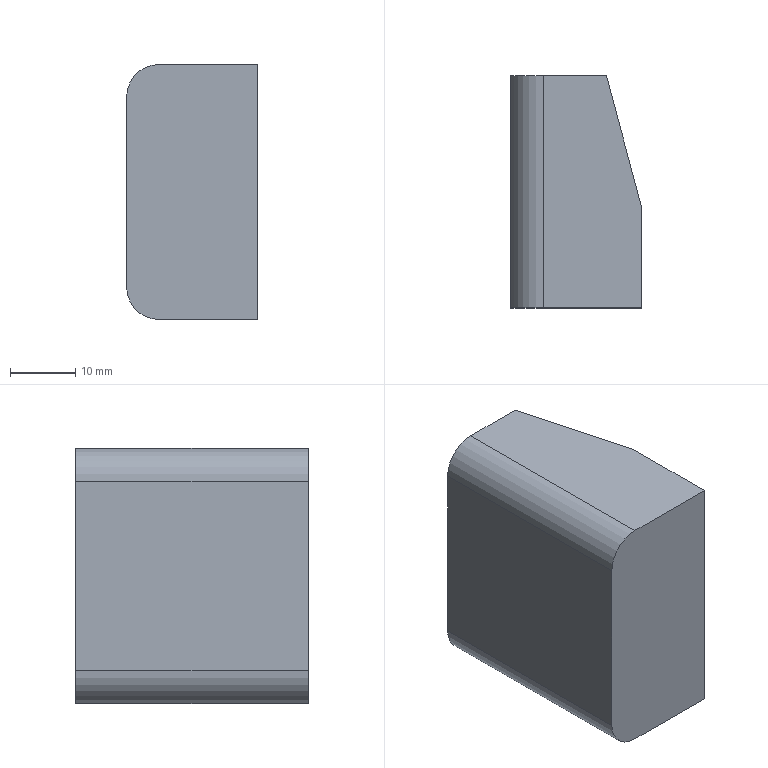Part | STEP file | 1 solid | 9 faces | box 20 x 35.5 x 39 mm | volume 25224 mm3 | plane 7 | cylinder 2 | commonest cylinder face diameters 10 x2
STEP:
#1=CARTESIAN_POINT('',(0.,0.,0.));
#2=DIRECTION('',(0.,0.,1.));
#3=DIRECTION('',(1.,0.,0.));
#4=AXIS2_PLACEMENT_3D('',#1,#2,#3);
#5=CARTESIAN_POINT('',(-257.863,50.,145.951));
#6=VERTEX_POINT('',#5);
#7=CARTESIAN_POINT('',(-252.863,50.,140.951));
#8=VERTEX_POINT('',#7);
#9=CARTESIAN_POINT('',(-252.863,50.,145.951));
#10=DIRECTION('',(0.,-1.,0.));
#11=DIRECTION('',(0.,0.,1.));
#12=AXIS2_PLACEMENT_3D('',#9,#10,#11);
#13=CIRCLE('',#12,5.);
#14=CARTESIAN_POINT('',(-252.863,-7.5,145.951));
#15=DIRECTION('',(0.,-1.,0.));
#16=DIRECTION('',(0.,0.,-1.));
#17=AXIS2_PLACEMENT_3D('',#14,#15,#16);
#18=CYLINDRICAL_SURFACE('',#17,5.);
#19=CARTESIAN_POINT('',(3.142,-57.5));
#20=DIRECTION('',(1.,0.));
#21=VECTOR('',#20,1.);
#22=LINE('',#19,#21);
#23=(GEOMETRIC_REPRESENTATION_CONTEXT(2)PARAMETRIC_REPRESENTATION_CONTEXT()REPRESENTATION_CONTEXT('',''));
#24=DEFINITIONAL_REPRESENTATION('',(#22),#23);
#25=PCURVE('',#18,#24);
#26=CARTESIAN_POINT('',(-72.862,50.,108.53));
#27=DIRECTION('',(0.,1.,0.));
#28=DIRECTION('',(0.,0.,1.));
#29=AXIS2_PLACEMENT_3D('',#26,#27,#28);
#30=PLANE('',#29);
#31=CARTESIAN_POINT('',(42.422,-180.));
#32=CARTESIAN_POINT('',(42.422,-188.66));
#33=CARTESIAN_POINT('',(34.922,-184.33));
#34=CARTESIAN_POINT('',(27.422,-180.));
#35=CARTESIAN_POINT('',(34.922,-175.67));
#36=CARTESIAN_POINT('',(42.422,-171.34));
#37=CARTESIAN_POINT('',(42.422,-180.));
#38=(BOUNDED_CURVE()B_SPLINE_CURVE(2,(#31,#32,#33,#34,#35,#36,#37),.UNSPECIFIED.,.T.,.F.)B_SPLINE_CURVE_WITH_KNOTS((1,2,2,2,2,1),(-2.094,0.,2.094,4.189,6.283,8.378),.UNSPECIFIED.)CURVE()GEOMETRIC_REPRESENTATION_ITEM()RATIONAL_B_SPLINE_CURVE((1.,0.5,1.,0.5,1.,0.5,1.))REPRESENTATION_ITEM(''));
#39=(GEOMETRIC_REPRESENTATION_CONTEXT(2)PARAMETRIC_REPRESENTATION_CONTEXT()REPRESENTATION_CONTEXT('',''));
#40=DEFINITIONAL_REPRESENTATION('',(#38),#39);
#41=PCURVE('',#30,#40);
#42=SURFACE_CURVE('',#13,(#25,#41),.PCURVE_S1.);
#43=EDGE_CURVE('',#6,#8,#42,.T.);
#44=ORIENTED_EDGE('',*,*,#43,.F.);
#45=CARTESIAN_POINT('',(-257.863,85.5,145.951));
#46=VERTEX_POINT('',#45);
#47=CARTESIAN_POINT('',(-257.863,-7.5,145.951));
#48=DIRECTION('',(0.,-1.,0.));
#49=VECTOR('',#48,1.);
#50=LINE('',#47,#49);
#51=CARTESIAN_POINT('',(4.712,0.));
#52=DIRECTION('',(0.,1.));
#53=VECTOR('',#52,1.);
#54=LINE('',#51,#53);
#55=(GEOMETRIC_REPRESENTATION_CONTEXT(2)PARAMETRIC_REPRESENTATION_CONTEXT()REPRESENTATION_CONTEXT('',''));
#56=DEFINITIONAL_REPRESENTATION('',(#54),#55);
#57=PCURVE('',#18,#56);
#58=CARTESIAN_POINT('',(-257.863,-7.5,140.951));
#59=DIRECTION('',(-1.,0.,0.));
#60=DIRECTION('',(0.,0.,1.));
#61=AXIS2_PLACEMENT_3D('',#58,#59,#60);
#62=PLANE('',#61);
#63=CARTESIAN_POINT('',(5.,0.));
#64=DIRECTION('',(0.,-1.));
#65=VECTOR('',#64,1.);
#66=LINE('',#63,#65);
#67=(GEOMETRIC_REPRESENTATION_CONTEXT(2)PARAMETRIC_REPRESENTATION_CONTEXT()REPRESENTATION_CONTEXT('',''));
#68=DEFINITIONAL_REPRESENTATION('',(#66),#67);
#69=PCURVE('',#62,#68);
#70=SURFACE_CURVE('',#50,(#57,#69),.PCURVE_S1.);
#71=EDGE_CURVE('',#46,#6,#70,.T.);
#72=ORIENTED_EDGE('',*,*,#71,.F.);
#73=CARTESIAN_POINT('',(-252.863,85.5,140.951));
#74=VERTEX_POINT('',#73);
#75=CARTESIAN_POINT('',(-252.863,85.5,145.951));
#76=DIRECTION('',(0.,1.,0.));
#77=DIRECTION('',(0.,0.,-1.));
#78=AXIS2_PLACEMENT_3D('',#75,#76,#77);
#79=CIRCLE('',#78,5.);
#80=CARTESIAN_POINT('',(6.283,-93.));
#81=DIRECTION('',(-1.,0.));
#82=VECTOR('',#81,1.);
#83=LINE('',#80,#82);
#84=(GEOMETRIC_REPRESENTATION_CONTEXT(2)PARAMETRIC_REPRESENTATION_CONTEXT()REPRESENTATION_CONTEXT('',''));
#85=DEFINITIONAL_REPRESENTATION('',(#83),#84);
#86=PCURVE('',#18,#85);
#87=CARTESIAN_POINT('',(-72.862,85.5,-363.47));
#88=DIRECTION('',(0.,-1.,0.));
#89=DIRECTION('',(0.,0.,-1.));
#90=AXIS2_PLACEMENT_3D('',#87,#88,#89);
#91=PLANE('',#90);
#92=CARTESIAN_POINT('',(-504.422,-180.));
#93=CARTESIAN_POINT('',(-504.422,-188.66));
#94=CARTESIAN_POINT('',(-511.922,-184.33));
#95=CARTESIAN_POINT('',(-519.422,-180.));
#96=CARTESIAN_POINT('',(-511.922,-175.67));
#97=CARTESIAN_POINT('',(-504.422,-171.34));
#98=CARTESIAN_POINT('',(-504.422,-180.));
#99=(BOUNDED_CURVE()B_SPLINE_CURVE(2,(#92,#93,#94,#95,#96,#97,#98),.UNSPECIFIED.,.T.,.F.)B_SPLINE_CURVE_WITH_KNOTS((1,2,2,2,2,1),(-2.094,0.,2.094,4.189,6.283,8.378),.UNSPECIFIED.)CURVE()GEOMETRIC_REPRESENTATION_ITEM()RATIONAL_B_SPLINE_CURVE((1.,0.5,1.,0.5,1.,0.5,1.))REPRESENTATION_ITEM(''));
#100=(GEOMETRIC_REPRESENTATION_CONTEXT(2)PARAMETRIC_REPRESENTATION_CONTEXT()REPRESENTATION_CONTEXT('',''));
#101=DEFINITIONAL_REPRESENTATION('',(#99),#100);
#102=PCURVE('',#91,#101);
#103=SURFACE_CURVE('',#79,(#86,#102),.PCURVE_S1.);
#104=EDGE_CURVE('',#74,#46,#103,.T.);
#105=ORIENTED_EDGE('',*,*,#104,.F.);
#106=CARTESIAN_POINT('',(-252.863,-7.5,140.951));
#107=DIRECTION('',(0.,1.,0.));
#108=VECTOR('',#107,1.);
#109=LINE('',#106,#108);
#110=CARTESIAN_POINT('',(6.283,0.));
#111=DIRECTION('',(0.,-1.));
#112=VECTOR('',#111,1.);
#113=LINE('',#110,#112);
#114=(GEOMETRIC_REPRESENTATION_CONTEXT(2)PARAMETRIC_REPRESENTATION_CONTEXT()REPRESENTATION_CONTEXT('',''));
#115=DEFINITIONAL_REPRESENTATION('',(#113),#114);
#116=PCURVE('',#18,#115);
#117=CARTESIAN_POINT('',(-240.363,-7.5,140.951));
#118=DIRECTION('',(0.,0.,-1.));
#119=DIRECTION('',(-1.,0.,0.));
#120=AXIS2_PLACEMENT_3D('',#117,#118,#119);
#121=PLANE('',#120);
#122=CARTESIAN_POINT('',(12.5,0.));
#123=DIRECTION('',(0.,1.));
#124=VECTOR('',#123,1.);
#125=LINE('',#122,#124);
#126=(GEOMETRIC_REPRESENTATION_CONTEXT(2)PARAMETRIC_REPRESENTATION_CONTEXT()REPRESENTATION_CONTEXT('',''));
#127=DEFINITIONAL_REPRESENTATION('',(#125),#126);
#128=PCURVE('',#121,#127);
#129=SURFACE_CURVE('',#109,(#116,#128),.PCURVE_S1.);
#130=EDGE_CURVE('',#8,#74,#129,.T.);
#131=ORIENTED_EDGE('',*,*,#130,.F.);
#132=EDGE_LOOP('',(#44,#72,#105,#131));
#133=FACE_BOUND('',#132,.T.);
#134=ADVANCED_FACE('',(#133),#18,.T.);
#135=CARTESIAN_POINT('',(-257.863,50.,174.951));
#136=VERTEX_POINT('',#135);
#137=CARTESIAN_POINT('',(-257.863,50.,140.951));
#138=DIRECTION('',(0.,0.,-1.));
#139=VECTOR('',#138,1.);
#140=LINE('',#137,#139);
#141=CARTESIAN_POINT('',(0.,57.5));
#142=DIRECTION('',(-1.,0.));
#143=VECTOR('',#142,1.);
#144=LINE('',#141,#143);
#145=(GEOMETRIC_REPRESENTATION_CONTEXT(2)PARAMETRIC_REPRESENTATION_CONTEXT()REPRESENTATION_CONTEXT('',''));
#146=DEFINITIONAL_REPRESENTATION('',(#144),#145);
#147=PCURVE('',#62,#146);
#148=CARTESIAN_POINT('',(32.422,-185.));
#149=DIRECTION('',(-1.,0.));
#150=VECTOR('',#149,1.);
#151=LINE('',#148,#150);
#152=(GEOMETRIC_REPRESENTATION_CONTEXT(2)PARAMETRIC_REPRESENTATION_CONTEXT()REPRESENTATION_CONTEXT('',''));
#153=DEFINITIONAL_REPRESENTATION('',(#151),#152);
#154=PCURVE('',#30,#153);
#155=SURFACE_CURVE('',#140,(#147,#154),.PCURVE_S1.);
#156=EDGE_CURVE('',#136,#6,#155,.T.);
#157=ORIENTED_EDGE('',*,*,#156,.F.);
#158=CARTESIAN_POINT('',(-257.863,85.5,174.951));
#159=VERTEX_POINT('',#158);
#160=CARTESIAN_POINT('',(-257.863,-7.5,174.951));
#161=DIRECTION('',(0.,1.,0.));
#162=VECTOR('',#161,1.);
#163=LINE('',#160,#162);
#164=CARTESIAN_POINT('',(34.,0.));
#165=DIRECTION('',(0.,1.));
#166=VECTOR('',#165,1.);
#167=LINE('',#164,#166);
#168=(GEOMETRIC_REPRESENTATION_CONTEXT(2)PARAMETRIC_REPRESENTATION_CONTEXT()REPRESENTATION_CONTEXT('',''));
#169=DEFINITIONAL_REPRESENTATION('',(#167),#168);
#170=PCURVE('',#62,#169);
#171=CARTESIAN_POINT('',(-252.863,-7.5,174.951));
#172=DIRECTION('',(0.,1.,0.));
#173=DIRECTION('',(0.,0.,1.));
#174=AXIS2_PLACEMENT_3D('',#171,#172,#173);
#175=CYLINDRICAL_SURFACE('',#174,5.);
#176=CARTESIAN_POINT('',(4.712,0.));
#177=DIRECTION('',(0.,1.));
#178=VECTOR('',#177,1.);
#179=LINE('',#176,#178);
#180=(GEOMETRIC_REPRESENTATION_CONTEXT(2)PARAMETRIC_REPRESENTATION_CONTEXT()REPRESENTATION_CONTEXT('',''));
#181=DEFINITIONAL_REPRESENTATION('',(#179),#180);
#182=PCURVE('',#175,#181);
#183=SURFACE_CURVE('',#163,(#170,#182),.PCURVE_S1.);
#184=EDGE_CURVE('',#136,#159,#183,.T.);
#185=ORIENTED_EDGE('',*,*,#184,.T.);
#186=CARTESIAN_POINT('',(-257.863,85.5,-363.47));
#187=DIRECTION('',(0.,0.,1.));
#188=VECTOR('',#187,1.);
#189=LINE('',#186,#188);
#190=CARTESIAN_POINT('',(-504.422,93.));
#191=DIRECTION('',(1.,0.));
#192=VECTOR('',#191,1.);
#193=LINE('',#190,#192);
#194=(GEOMETRIC_REPRESENTATION_CONTEXT(2)PARAMETRIC_REPRESENTATION_CONTEXT()REPRESENTATION_CONTEXT('',''));
#195=DEFINITIONAL_REPRESENTATION('',(#193),#194);
#196=PCURVE('',#62,#195);
#197=CARTESIAN_POINT('',(0.,-185.));
#198=DIRECTION('',(-1.,0.));
#199=VECTOR('',#198,1.);
#200=LINE('',#197,#199);
#201=(GEOMETRIC_REPRESENTATION_CONTEXT(2)PARAMETRIC_REPRESENTATION_CONTEXT()REPRESENTATION_CONTEXT('',''));
#202=DEFINITIONAL_REPRESENTATION('',(#200),#201);
#203=PCURVE('',#91,#202);
#204=SURFACE_CURVE('',#189,(#196,#203),.PCURVE_S1.);
#205=EDGE_CURVE('',#46,#159,#204,.T.);
#206=ORIENTED_EDGE('',*,*,#205,.F.);
#207=ORIENTED_EDGE('',*,*,#71,.T.);
#208=EDGE_LOOP('',(#157,#185,#206,#207));
#209=FACE_BOUND('',#208,.T.);
#210=ADVANCED_FACE('',(#209),#62,.T.);
#211=CARTESIAN_POINT('',(-252.863,50.,179.951));
#212=VERTEX_POINT('',#211);
#213=CARTESIAN_POINT('',(-252.863,50.,174.951));
#214=DIRECTION('',(0.,-1.,0.));
#215=DIRECTION('',(0.,0.,1.));
#216=AXIS2_PLACEMENT_3D('',#213,#214,#215);
#217=CIRCLE('',#216,5.);
#218=CARTESIAN_POINT('',(6.283,57.5));
#219=DIRECTION('',(-1.,0.));
#220=VECTOR('',#219,1.);
#221=LINE('',#218,#220);
#222=(GEOMETRIC_REPRESENTATION_CONTEXT(2)PARAMETRIC_REPRESENTATION_CONTEXT()REPRESENTATION_CONTEXT('',''));
#223=DEFINITIONAL_REPRESENTATION('',(#221),#222);
#224=PCURVE('',#175,#223);
#225=CARTESIAN_POINT('',(71.422,-180.));
#226=CARTESIAN_POINT('',(71.422,-188.66));
#227=CARTESIAN_POINT('',(63.922,-184.33));
#228=CARTESIAN_POINT('',(56.422,-180.));
#229=CARTESIAN_POINT('',(63.922,-175.67));
#230=CARTESIAN_POINT('',(71.422,-171.34));
#231=CARTESIAN_POINT('',(71.422,-180.));
#232=(BOUNDED_CURVE()B_SPLINE_CURVE(2,(#225,#226,#227,#228,#229,#230,#231),.UNSPECIFIED.,.T.,.F.)B_SPLINE_CURVE_WITH_KNOTS((1,2,2,2,2,1),(-2.094,0.,2.094,4.189,6.283,8.378),.UNSPECIFIED.)CURVE()GEOMETRIC_REPRESENTATION_ITEM()RATIONAL_B_SPLINE_CURVE((1.,0.5,1.,0.5,1.,0.5,1.))REPRESENTATION_ITEM(''));
#233=(GEOMETRIC_REPRESENTATION_CONTEXT(2)PARAMETRIC_REPRESENTATION_CONTEXT()REPRESENTATION_CONTEXT('',''));
#234=DEFINITIONAL_REPRESENTATION('',(#232),#233);
#235=PCURVE('',#30,#234);
#236=SURFACE_CURVE('',#217,(#224,#235),.PCURVE_S1.);
#237=EDGE_CURVE('',#212,#136,#236,.T.);
#238=ORIENTED_EDGE('',*,*,#237,.F.);
#239=CARTESIAN_POINT('',(-252.863,85.5,179.951));
#240=VERTEX_POINT('',#239);
#241=CARTESIAN_POINT('',(-252.863,-7.5,179.951));
#242=DIRECTION('',(0.,-1.,0.));
#243=VECTOR('',#242,1.);
#244=LINE('',#241,#243);
#245=CARTESIAN_POINT('',(6.283,0.));
#246=DIRECTION('',(0.,-1.));
#247=VECTOR('',#246,1.);
#248=LINE('',#245,#247);
#249=(GEOMETRIC_REPRESENTATION_CONTEXT(2)PARAMETRIC_REPRESENTATION_CONTEXT()REPRESENTATION_CONTEXT('',''));
#250=DEFINITIONAL_REPRESENTATION('',(#248),#249);
#251=PCURVE('',#175,#250);
#252=CARTESIAN_POINT('',(-240.363,-7.5,179.951));
#253=DIRECTION('',(0.,0.,1.));
#254=DIRECTION('',(1.,0.,0.));
#255=AXIS2_PLACEMENT_3D('',#252,#253,#254);
#256=PLANE('',#255);
#257=CARTESIAN_POINT('',(-12.5,0.));
#258=DIRECTION('',(0.,-1.));
#259=VECTOR('',#258,1.);
#260=LINE('',#257,#259);
#261=(GEOMETRIC_REPRESENTATION_CONTEXT(2)PARAMETRIC_REPRESENTATION_CONTEXT()REPRESENTATION_CONTEXT('',''));
#262=DEFINITIONAL_REPRESENTATION('',(#260),#261);
#263=PCURVE('',#256,#262);
#264=SURFACE_CURVE('',#244,(#251,#263),.PCURVE_S1.);
#265=EDGE_CURVE('',#240,#212,#264,.T.);
#266=ORIENTED_EDGE('',*,*,#265,.F.);
#267=CARTESIAN_POINT('',(-252.863,85.5,174.951));
#268=DIRECTION('',(0.,1.,0.));
#269=DIRECTION('',(0.,0.,-1.));
#270=AXIS2_PLACEMENT_3D('',#267,#268,#269);
#271=CIRCLE('',#270,5.);
#272=CARTESIAN_POINT('',(3.142,93.));
#273=DIRECTION('',(1.,0.));
#274=VECTOR('',#273,1.);
#275=LINE('',#272,#274);
#276=(GEOMETRIC_REPRESENTATION_CONTEXT(2)PARAMETRIC_REPRESENTATION_CONTEXT()REPRESENTATION_CONTEXT('',''));
#277=DEFINITIONAL_REPRESENTATION('',(#275),#276);
#278=PCURVE('',#175,#277);
#279=CARTESIAN_POINT('',(-533.422,-180.));
#280=CARTESIAN_POINT('',(-533.422,-188.66));
#281=CARTESIAN_POINT('',(-540.922,-184.33));
#282=CARTESIAN_POINT('',(-548.422,-180.));
#283=CARTESIAN_POINT('',(-540.922,-175.67));
#284=CARTESIAN_POINT('',(-533.422,-171.34));
#285=CARTESIAN_POINT('',(-533.422,-180.));
#286=(BOUNDED_CURVE()B_SPLINE_CURVE(2,(#279,#280,#281,#282,#283,#284,#285),.UNSPECIFIED.,.T.,.F.)B_SPLINE_CURVE_WITH_KNOTS((1,2,2,2,2,1),(-2.094,0.,2.094,4.189,6.283,8.378),.UNSPECIFIED.)CURVE()GEOMETRIC_REPRESENTATION_ITEM()RATIONAL_B_SPLINE_CURVE((1.,0.5,1.,0.5,1.,0.5,1.))REPRESENTATION_ITEM(''));
#287=(GEOMETRIC_REPRESENTATION_CONTEXT(2)PARAMETRIC_REPRESENTATION_CONTEXT()REPRESENTATION_CONTEXT('',''));
#288=DEFINITIONAL_REPRESENTATION('',(#286),#287);
#289=PCURVE('',#91,#288);
#290=SURFACE_CURVE('',#271,(#278,#289),.PCURVE_S1.);
#291=EDGE_CURVE('',#159,#240,#290,.T.);
#292=ORIENTED_EDGE('',*,*,#291,.F.);
#293=ORIENTED_EDGE('',*,*,#184,.F.);
#294=EDGE_LOOP('',(#238,#266,#292,#293));
#295=FACE_BOUND('',#294,.T.);
#296=ADVANCED_FACE('',(#295),#175,.T.);
#297=CARTESIAN_POINT('',(-237.863,50.,140.951));
#298=VERTEX_POINT('',#297);
#299=CARTESIAN_POINT('',(-240.363,50.,140.951));
#300=DIRECTION('',(1.,0.,0.));
#301=VECTOR('',#300,1.);
#302=LINE('',#299,#301);
#303=CARTESIAN_POINT('',(32.422,-167.5));
#304=DIRECTION('',(0.,1.));
#305=VECTOR('',#304,1.);
#306=LINE('',#303,#305);
#307=(GEOMETRIC_REPRESENTATION_CONTEXT(2)PARAMETRIC_REPRESENTATION_CONTEXT()REPRESENTATION_CONTEXT('',''));
#308=DEFINITIONAL_REPRESENTATION('',(#306),#307);
#309=PCURVE('',#30,#308);
#310=CARTESIAN_POINT('',(0.,57.5));
#311=DIRECTION('',(-1.,0.));
#312=VECTOR('',#311,1.);
#313=LINE('',#310,#312);
#314=(GEOMETRIC_REPRESENTATION_CONTEXT(2)PARAMETRIC_REPRESENTATION_CONTEXT()REPRESENTATION_CONTEXT('',''));
#315=DEFINITIONAL_REPRESENTATION('',(#313),#314);
#316=PCURVE('',#121,#315);
#317=SURFACE_CURVE('',#302,(#309,#316),.PCURVE_S1.);
#318=EDGE_CURVE('',#8,#298,#317,.T.);
#319=ORIENTED_EDGE('',*,*,#318,.T.);
#320=CARTESIAN_POINT('',(-237.863,50.,179.951));
#321=VERTEX_POINT('',#320);
#322=CARTESIAN_POINT('',(-237.863,50.,108.53));
#323=DIRECTION('',(0.,0.,1.));
#324=VECTOR('',#323,1.);
#325=LINE('',#322,#324);
#326=CARTESIAN_POINT('',(0.,-165.));
#327=DIRECTION('',(1.,0.));
#328=VECTOR('',#327,1.);
#329=LINE('',#326,#328);
#330=(GEOMETRIC_REPRESENTATION_CONTEXT(2)PARAMETRIC_REPRESENTATION_CONTEXT()REPRESENTATION_CONTEXT('',''));
#331=DEFINITIONAL_REPRESENTATION('',(#329),#330);
#332=PCURVE('',#30,#331);
#333=CARTESIAN_POINT('',(-237.863,67.75,160.451));
#334=DIRECTION('',(-1.,0.,0.));
#335=DIRECTION('',(0.,0.,1.));
#336=AXIS2_PLACEMENT_3D('',#333,#334,#335);
#337=PLANE('',#336);
#338=CARTESIAN_POINT('',(-51.922,-17.75));
#339=DIRECTION('',(1.,0.));
#340=VECTOR('',#339,1.);
#341=LINE('',#338,#340);
#342=(GEOMETRIC_REPRESENTATION_CONTEXT(2)PARAMETRIC_REPRESENTATION_CONTEXT()REPRESENTATION_CONTEXT('',''));
#343=DEFINITIONAL_REPRESENTATION('',(#341),#342);
#344=PCURVE('',#337,#343);
#345=SURFACE_CURVE('',#325,(#332,#344),.PCURVE_S1.);
#346=EDGE_CURVE('',#298,#321,#345,.T.);
#347=ORIENTED_EDGE('',*,*,#346,.T.);
#348=CARTESIAN_POINT('',(-240.363,50.,179.951));
#349=DIRECTION('',(-1.,0.,0.));
#350=VECTOR('',#349,1.);
#351=LINE('',#348,#350);
#352=CARTESIAN_POINT('',(71.422,-167.5));
#353=DIRECTION('',(0.,-1.));
#354=VECTOR('',#353,1.);
#355=LINE('',#352,#354);
#356=(GEOMETRIC_REPRESENTATION_CONTEXT(2)PARAMETRIC_REPRESENTATION_CONTEXT()REPRESENTATION_CONTEXT('',''));
#357=DEFINITIONAL_REPRESENTATION('',(#355),#356);
#358=PCURVE('',#30,#357);
#359=CARTESIAN_POINT('',(0.,57.5));
#360=DIRECTION('',(-1.,0.));
#361=VECTOR('',#360,1.);
#362=LINE('',#359,#361);
#363=(GEOMETRIC_REPRESENTATION_CONTEXT(2)PARAMETRIC_REPRESENTATION_CONTEXT()REPRESENTATION_CONTEXT('',''));
#364=DEFINITIONAL_REPRESENTATION('',(#362),#363);
#365=PCURVE('',#256,#364);
#366=SURFACE_CURVE('',#351,(#358,#365),.PCURVE_S1.);
#367=EDGE_CURVE('',#321,#212,#366,.T.);
#368=ORIENTED_EDGE('',*,*,#367,.T.);
#369=ORIENTED_EDGE('',*,*,#237,.T.);
#370=ORIENTED_EDGE('',*,*,#156,.T.);
#371=ORIENTED_EDGE('',*,*,#43,.T.);
#372=EDGE_LOOP('',(#319,#347,#368,#369,#370,#371));
#373=FACE_BOUND('',#372,.T.);
#374=ADVANCED_FACE('',(#373),#30,.F.);
#375=CARTESIAN_POINT('',(-237.863,65.523,140.951));
#376=VERTEX_POINT('',#375);
#377=CARTESIAN_POINT('',(-243.215,85.5,140.951));
#378=VERTEX_POINT('',#377);
#379=CARTESIAN_POINT('',(-219.774,-1.983,140.951));
#380=DIRECTION('',(-0.2588,0.9659,0.));
#381=VECTOR('',#380,1.);
#382=LINE('',#379,#381);
#383=CARTESIAN_POINT('',(-20.588,5.517));
#384=DIRECTION('',(0.2588,0.9659));
#385=VECTOR('',#384,1.);
#386=LINE('',#383,#385);
#387=(GEOMETRIC_REPRESENTATION_CONTEXT(2)PARAMETRIC_REPRESENTATION_CONTEXT()REPRESENTATION_CONTEXT('',''));
#388=DEFINITIONAL_REPRESENTATION('',(#386),#387);
#389=PCURVE('',#121,#388);
#390=CARTESIAN_POINT('',(-242.522,82.912,180.451));
#391=DIRECTION('',(-0.9659,-0.2588,0.));
#392=DIRECTION('',(0.2588,-0.9659,0.));
#393=AXIS2_PLACEMENT_3D('',#390,#391,#392);
#394=PLANE('',#393);
#395=CARTESIAN_POINT('',(87.89,-39.5));
#396=DIRECTION('',(-1.,0.));
#397=VECTOR('',#396,1.);
#398=LINE('',#395,#397);
#399=(GEOMETRIC_REPRESENTATION_CONTEXT(2)PARAMETRIC_REPRESENTATION_CONTEXT()REPRESENTATION_CONTEXT('',''));
#400=DEFINITIONAL_REPRESENTATION('',(#398),#399);
#401=PCURVE('',#394,#400);
#402=SURFACE_CURVE('',#382,(#389,#401),.PCURVE_S1.);
#403=EDGE_CURVE('',#376,#378,#402,.T.);
#404=ORIENTED_EDGE('',*,*,#403,.F.);
#405=CARTESIAN_POINT('',(-237.863,-7.5,140.951));
#406=DIRECTION('',(0.,1.,0.));
#407=VECTOR('',#406,1.);
#408=LINE('',#405,#407);
#409=CARTESIAN_POINT('',(-2.5,0.));
#410=DIRECTION('',(0.,1.));
#411=VECTOR('',#410,1.);
#412=LINE('',#409,#411);
#413=(GEOMETRIC_REPRESENTATION_CONTEXT(2)PARAMETRIC_REPRESENTATION_CONTEXT()REPRESENTATION_CONTEXT('',''));
#414=DEFINITIONAL_REPRESENTATION('',(#412),#413);
#415=PCURVE('',#121,#414);
#416=CARTESIAN_POINT('',(-19.5,-75.25));
#417=DIRECTION('',(0.,1.));
#418=VECTOR('',#417,1.);
#419=LINE('',#416,#418);
#420=(GEOMETRIC_REPRESENTATION_CONTEXT(2)PARAMETRIC_REPRESENTATION_CONTEXT()REPRESENTATION_CONTEXT('',''));
#421=DEFINITIONAL_REPRESENTATION('',(#419),#420);
#422=PCURVE('',#337,#421);
#423=SURFACE_CURVE('',#408,(#415,#422),.PCURVE_S1.);
#424=EDGE_CURVE('',#298,#376,#423,.T.);
#425=ORIENTED_EDGE('',*,*,#424,.F.);
#426=ORIENTED_EDGE('',*,*,#318,.F.);
#427=ORIENTED_EDGE('',*,*,#130,.T.);
#428=CARTESIAN_POINT('',(-72.862,85.5,140.951));
#429=DIRECTION('',(-1.,0.,0.));
#430=VECTOR('',#429,1.);
#431=LINE('',#428,#430);
#432=CARTESIAN_POINT('',(-167.5,93.));
#433=DIRECTION('',(1.,0.));
#434=VECTOR('',#433,1.);
#435=LINE('',#432,#434);
#436=(GEOMETRIC_REPRESENTATION_CONTEXT(2)PARAMETRIC_REPRESENTATION_CONTEXT()REPRESENTATION_CONTEXT('',''));
#437=DEFINITIONAL_REPRESENTATION('',(#435),#436);
#438=PCURVE('',#121,#437);
#439=CARTESIAN_POINT('',(-504.422,0.));
#440=DIRECTION('',(0.,-1.));
#441=VECTOR('',#440,1.);
#442=LINE('',#439,#441);
#443=(GEOMETRIC_REPRESENTATION_CONTEXT(2)PARAMETRIC_REPRESENTATION_CONTEXT()REPRESENTATION_CONTEXT('',''));
#444=DEFINITIONAL_REPRESENTATION('',(#442),#443);
#445=PCURVE('',#91,#444);
#446=SURFACE_CURVE('',#431,(#438,#445),.PCURVE_S1.);
#447=EDGE_CURVE('',#378,#74,#446,.T.);
#448=ORIENTED_EDGE('',*,*,#447,.F.);
#449=EDGE_LOOP('',(#404,#425,#426,#427,#448));
#450=FACE_BOUND('',#449,.T.);
#451=ADVANCED_FACE('',(#450),#121,.T.);
#452=CARTESIAN_POINT('',(-243.215,85.5,179.951));
#453=VERTEX_POINT('',#452);
#454=CARTESIAN_POINT('',(-243.215,85.5,-363.47));
#455=DIRECTION('',(0.,0.,1.));
#456=VECTOR('',#455,1.);
#457=LINE('',#454,#456);
#458=CARTESIAN_POINT('',(0.,-170.353));
#459=DIRECTION('',(-1.,0.));
#460=VECTOR('',#459,1.);
#461=LINE('',#458,#460);
#462=(GEOMETRIC_REPRESENTATION_CONTEXT(2)PARAMETRIC_REPRESENTATION_CONTEXT()REPRESENTATION_CONTEXT('',''));
#463=DEFINITIONAL_REPRESENTATION('',(#461),#462);
#464=PCURVE('',#91,#463);
#465=CARTESIAN_POINT('',(-2.679,-543.922));
#466=DIRECTION('',(0.,1.));
#467=VECTOR('',#466,1.);
#468=LINE('',#465,#467);
#469=(GEOMETRIC_REPRESENTATION_CONTEXT(2)PARAMETRIC_REPRESENTATION_CONTEXT()REPRESENTATION_CONTEXT('',''));
#470=DEFINITIONAL_REPRESENTATION('',(#468),#469);
#471=PCURVE('',#394,#470);
#472=SURFACE_CURVE('',#457,(#464,#471),.PCURVE_S1.);
#473=EDGE_CURVE('',#378,#453,#472,.T.);
#474=ORIENTED_EDGE('',*,*,#473,.F.);
#475=ORIENTED_EDGE('',*,*,#447,.T.);
#476=ORIENTED_EDGE('',*,*,#104,.T.);
#477=ORIENTED_EDGE('',*,*,#205,.T.);
#478=ORIENTED_EDGE('',*,*,#291,.T.);
#479=CARTESIAN_POINT('',(-72.862,85.5,179.951));
#480=DIRECTION('',(1.,0.,0.));
#481=VECTOR('',#480,1.);
#482=LINE('',#479,#481);
#483=CARTESIAN_POINT('',(-543.422,0.));
#484=DIRECTION('',(0.,1.));
#485=VECTOR('',#484,1.);
#486=LINE('',#483,#485);
#487=(GEOMETRIC_REPRESENTATION_CONTEXT(2)PARAMETRIC_REPRESENTATION_CONTEXT()REPRESENTATION_CONTEXT('',''));
#488=DEFINITIONAL_REPRESENTATION('',(#486),#487);
#489=PCURVE('',#91,#488);
#490=CARTESIAN_POINT('',(167.5,93.));
#491=DIRECTION('',(1.,0.));
#492=VECTOR('',#491,1.);
#493=LINE('',#490,#492);
#494=(GEOMETRIC_REPRESENTATION_CONTEXT(2)PARAMETRIC_REPRESENTATION_CONTEXT()REPRESENTATION_CONTEXT('',''));
#495=DEFINITIONAL_REPRESENTATION('',(#493),#494);
#496=PCURVE('',#256,#495);
#497=SURFACE_CURVE('',#482,(#489,#496),.PCURVE_S1.);
#498=EDGE_CURVE('',#240,#453,#497,.T.);
#499=ORIENTED_EDGE('',*,*,#498,.T.);
#500=EDGE_LOOP('',(#474,#475,#476,#477,#478,#499));
#501=FACE_BOUND('',#500,.T.);
#502=ADVANCED_FACE('',(#501),#91,.F.);
#503=CARTESIAN_POINT('',(-237.863,65.523,179.951));
#504=VERTEX_POINT('',#503);
#505=CARTESIAN_POINT('',(-219.774,-1.983,179.951));
#506=DIRECTION('',(0.2588,-0.9659,0.));
#507=VECTOR('',#506,1.);
#508=LINE('',#505,#507);
#509=CARTESIAN_POINT('',(20.588,5.517));
#510=DIRECTION('',(0.2588,-0.9659));
#511=VECTOR('',#510,1.);
#512=LINE('',#509,#511);
#513=(GEOMETRIC_REPRESENTATION_CONTEXT(2)PARAMETRIC_REPRESENTATION_CONTEXT()REPRESENTATION_CONTEXT('',''));
#514=DEFINITIONAL_REPRESENTATION('',(#512),#513);
#515=PCURVE('',#256,#514);
#516=CARTESIAN_POINT('',(87.89,-0.5));
#517=DIRECTION('',(1.,0.));
#518=VECTOR('',#517,1.);
#519=LINE('',#516,#518);
#520=(GEOMETRIC_REPRESENTATION_CONTEXT(2)PARAMETRIC_REPRESENTATION_CONTEXT()REPRESENTATION_CONTEXT('',''));
#521=DEFINITIONAL_REPRESENTATION('',(#519),#520);
#522=PCURVE('',#394,#521);
#523=SURFACE_CURVE('',#508,(#515,#522),.PCURVE_S1.);
#524=EDGE_CURVE('',#453,#504,#523,.T.);
#525=ORIENTED_EDGE('',*,*,#524,.F.);
#526=ORIENTED_EDGE('',*,*,#498,.F.);
#527=ORIENTED_EDGE('',*,*,#265,.T.);
#528=ORIENTED_EDGE('',*,*,#367,.F.);
#529=CARTESIAN_POINT('',(-237.863,-7.5,179.951));
#530=DIRECTION('',(0.,-1.,0.));
#531=VECTOR('',#530,1.);
#532=LINE('',#529,#531);
#533=CARTESIAN_POINT('',(2.5,0.));
#534=DIRECTION('',(0.,-1.));
#535=VECTOR('',#534,1.);
#536=LINE('',#533,#535);
#537=(GEOMETRIC_REPRESENTATION_CONTEXT(2)PARAMETRIC_REPRESENTATION_CONTEXT()REPRESENTATION_CONTEXT('',''));
#538=DEFINITIONAL_REPRESENTATION('',(#536),#537);
#539=PCURVE('',#256,#538);
#540=CARTESIAN_POINT('',(19.5,-75.25));
#541=DIRECTION('',(0.,-1.));
#542=VECTOR('',#541,1.);
#543=LINE('',#540,#542);
#544=(GEOMETRIC_REPRESENTATION_CONTEXT(2)PARAMETRIC_REPRESENTATION_CONTEXT()REPRESENTATION_CONTEXT('',''));
#545=DEFINITIONAL_REPRESENTATION('',(#543),#544);
#546=PCURVE('',#337,#545);
#547=SURFACE_CURVE('',#532,(#539,#546),.PCURVE_S1.);
#548=EDGE_CURVE('',#504,#321,#547,.T.);
#549=ORIENTED_EDGE('',*,*,#548,.F.);
#550=EDGE_LOOP('',(#525,#526,#527,#528,#549));
#551=FACE_BOUND('',#550,.T.);
#552=ADVANCED_FACE('',(#551),#256,.T.);
#553=ORIENTED_EDGE('',*,*,#424,.T.);
#554=CARTESIAN_POINT('',(-237.863,65.523,160.451));
#555=DIRECTION('',(0.,0.,1.));
#556=VECTOR('',#555,1.);
#557=LINE('',#554,#556);
#558=CARTESIAN_POINT('',(0.,-2.227));
#559=DIRECTION('',(1.,0.));
#560=VECTOR('',#559,1.);
#561=LINE('',#558,#560);
#562=(GEOMETRIC_REPRESENTATION_CONTEXT(2)PARAMETRIC_REPRESENTATION_CONTEXT()REPRESENTATION_CONTEXT('',''));
#563=DEFINITIONAL_REPRESENTATION('',(#561),#562);
#564=PCURVE('',#337,#563);
#565=CARTESIAN_POINT('',(18.002,-20.));
#566=DIRECTION('',(0.,1.));
#567=VECTOR('',#566,1.);
#568=LINE('',#565,#567);
#569=(GEOMETRIC_REPRESENTATION_CONTEXT(2)PARAMETRIC_REPRESENTATION_CONTEXT()REPRESENTATION_CONTEXT('',''));
#570=DEFINITIONAL_REPRESENTATION('',(#568),#569);
#571=PCURVE('',#394,#570);
#572=SURFACE_CURVE('',#557,(#564,#571),.PCURVE_S1.);
#573=EDGE_CURVE('',#376,#504,#572,.T.);
#574=ORIENTED_EDGE('',*,*,#573,.T.);
#575=ORIENTED_EDGE('',*,*,#548,.T.);
#576=ORIENTED_EDGE('',*,*,#346,.F.);
#577=EDGE_LOOP('',(#553,#574,#575,#576));
#578=FACE_BOUND('',#577,.T.);
#579=ADVANCED_FACE('',(#578),#337,.F.);
#580=ORIENTED_EDGE('',*,*,#403,.T.);
#581=ORIENTED_EDGE('',*,*,#473,.T.);
#582=ORIENTED_EDGE('',*,*,#524,.T.);
#583=ORIENTED_EDGE('',*,*,#573,.F.);
#584=EDGE_LOOP('',(#580,#581,#582,#583));
#585=FACE_BOUND('',#584,.T.);
#586=ADVANCED_FACE('',(#585),#394,.F.);
#587=CLOSED_SHELL('',(#134,#210,#296,#374,#451,#502,#552,#579,#586));
#588=MANIFOLD_SOLID_BREP('',#587);
#589=(LENGTH_UNIT()NAMED_UNIT(*)SI_UNIT(.MILLI.,.METRE.));
#590=UNCERTAINTY_MEASURE_WITH_UNIT(LENGTH_MEASURE(0.0000001),#589,'','');
#591=(NAMED_UNIT(*)PLANE_ANGLE_UNIT()SI_UNIT($,.RADIAN.));
#592=(NAMED_UNIT(*)SI_UNIT($,.STERADIAN.)SOLID_ANGLE_UNIT());
#593=(GEOMETRIC_REPRESENTATION_CONTEXT(3)GLOBAL_UNCERTAINTY_ASSIGNED_CONTEXT((#590))GLOBAL_UNIT_ASSIGNED_CONTEXT((#589,#591,#592))REPRESENTATION_CONTEXT('',''));
#594=ADVANCED_BREP_SHAPE_REPRESENTATION('',(#4,#588),#593);